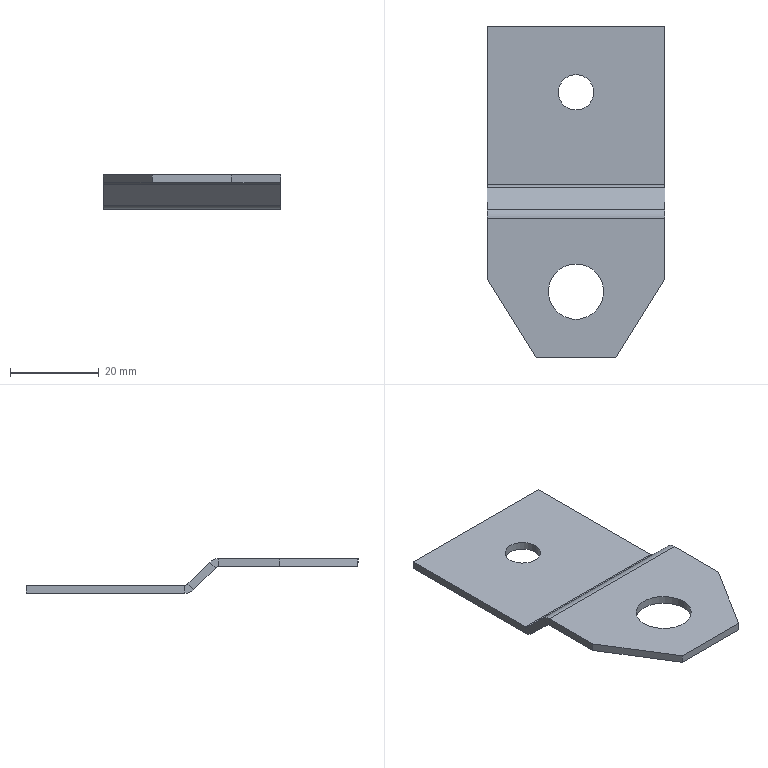Part | SolidWorks | features FlatPattern 1, Jog 1, SMBaseFlange 1, SheetMetal 1 | 1 solid | 28 faces | box 40 x 75 x 7.8 mm | volume 4907 mm3 | plane 20 | cylinder 8 | commonest cylinder face diameters 2 x2 5.6 x2 8 x2 12.5 x2
STEP:
#1=CARTESIAN_POINT('',(573.75,-25.,7.8));
#2=VERTEX_POINT('',#1);
#3=CARTESIAN_POINT('',(586.25,-25.,7.8));
#4=VERTEX_POINT('',#3);
#5=CARTESIAN_POINT('',(580.,-25.,7.8));
#6=DIRECTION('',(0.,0.,1.));
#7=DIRECTION('',(1.,0.,0.));
#8=AXIS2_PLACEMENT_3D('',#5,#6,#7);
#9=CIRCLE('',#8,6.25);
#10=EDGE_CURVE('',#2,#4,#9,.T.);
#11=ORIENTED_EDGE('',*,*,#10,.T.);
#12=CARTESIAN_POINT('',(586.25,-25.,6.));
#13=VERTEX_POINT('',#12);
#14=CARTESIAN_POINT('',(586.25,-25.,7.8));
#15=DIRECTION('',(0.,0.,-1.));
#16=VECTOR('',#15,1000.);
#17=LINE('',#14,#16);
#18=EDGE_CURVE('',#4,#13,#17,.T.);
#19=ORIENTED_EDGE('',*,*,#18,.T.);
#20=CARTESIAN_POINT('',(573.75,-25.,6.));
#21=VERTEX_POINT('',#20);
#22=CARTESIAN_POINT('',(580.,-25.,6.));
#23=DIRECTION('',(0.,0.,1.));
#24=DIRECTION('',(1.,0.,0.));
#25=AXIS2_PLACEMENT_3D('',#22,#23,#24);
#26=CIRCLE('',#25,6.25);
#27=EDGE_CURVE('',#21,#13,#26,.T.);
#28=ORIENTED_EDGE('',*,*,#27,.F.);
#29=CARTESIAN_POINT('',(573.75,-25.,7.8));
#30=DIRECTION('',(0.,0.,-1.));
#31=VECTOR('',#30,1000.);
#32=LINE('',#29,#31);
#33=EDGE_CURVE('',#2,#21,#32,.T.);
#34=ORIENTED_EDGE('',*,*,#33,.F.);
#35=EDGE_LOOP('',(#11,#19,#28,#34));
#36=FACE_OUTER_BOUND('',#35,.T.);
#37=CARTESIAN_POINT('',(580.,-25.,7.8));
#38=DIRECTION('',(0.,0.,-1.));
#39=DIRECTION('',(-1.,0.,0.));
#40=AXIS2_PLACEMENT_3D('',#37,#38,#39);
#41=CYLINDRICAL_SURFACE('',#40,6.25);
#42=ADVANCED_FACE('',(#36),#41,.F.);
#43=CARTESIAN_POINT('',(576.,20.,1.8));
#44=VERTEX_POINT('',#43);
#45=CARTESIAN_POINT('',(584.,20.,1.8));
#46=VERTEX_POINT('',#45);
#47=CARTESIAN_POINT('',(580.,20.,1.8));
#48=DIRECTION('',(0.,0.,1.));
#49=DIRECTION('',(1.,0.,0.));
#50=AXIS2_PLACEMENT_3D('',#47,#48,#49);
#51=CIRCLE('',#50,4.);
#52=EDGE_CURVE('',#44,#46,#51,.T.);
#53=ORIENTED_EDGE('',*,*,#52,.T.);
#54=CARTESIAN_POINT('',(584.,20.,0.));
#55=VERTEX_POINT('',#54);
#56=CARTESIAN_POINT('',(584.,20.,1.8));
#57=DIRECTION('',(0.,0.,-1.));
#58=VECTOR('',#57,1000.);
#59=LINE('',#56,#58);
#60=EDGE_CURVE('',#46,#55,#59,.T.);
#61=ORIENTED_EDGE('',*,*,#60,.T.);
#62=CARTESIAN_POINT('',(576.,20.,0.));
#63=VERTEX_POINT('',#62);
#64=CARTESIAN_POINT('',(580.,20.,0.));
#65=DIRECTION('',(0.,0.,1.));
#66=DIRECTION('',(1.,0.,0.));
#67=AXIS2_PLACEMENT_3D('',#64,#65,#66);
#68=CIRCLE('',#67,4.);
#69=EDGE_CURVE('',#63,#55,#68,.T.);
#70=ORIENTED_EDGE('',*,*,#69,.F.);
#71=CARTESIAN_POINT('',(576.,20.,1.8));
#72=DIRECTION('',(0.,0.,-1.));
#73=VECTOR('',#72,1000.);
#74=LINE('',#71,#73);
#75=EDGE_CURVE('',#44,#63,#74,.T.);
#76=ORIENTED_EDGE('',*,*,#75,.F.);
#77=EDGE_LOOP('',(#53,#61,#70,#76));
#78=FACE_OUTER_BOUND('',#77,.T.);
#79=CARTESIAN_POINT('',(580.,20.,1.8));
#80=DIRECTION('',(0.,0.,-1.));
#81=DIRECTION('',(-1.,0.,0.));
#82=AXIS2_PLACEMENT_3D('',#79,#80,#81);
#83=CYLINDRICAL_SURFACE('',#82,4.);
#84=ADVANCED_FACE('',(#78),#83,.F.);
#85=CARTESIAN_POINT('',(600.,-6.475,6.98));
#86=VERTEX_POINT('',#85);
#87=CARTESIAN_POINT('',(600.,-1.588,2.093));
#88=VERTEX_POINT('',#87);
#89=CARTESIAN_POINT('',(600.,24.729,-24.224));
#90=DIRECTION('',(0.,0.7071,-0.7071));
#91=VECTOR('',#90,1000.);
#92=LINE('',#89,#91);
#93=EDGE_CURVE('',#86,#88,#92,.T.);
#94=ORIENTED_EDGE('',*,*,#93,.F.);
#95=CARTESIAN_POINT('',(600.,-7.748,5.707));
#96=VERTEX_POINT('',#95);
#97=CARTESIAN_POINT('',(600.,-6.475,6.98));
#98=DIRECTION('',(0.,-0.7071,-0.7071));
#99=VECTOR('',#98,1000.);
#100=LINE('',#97,#99);
#101=EDGE_CURVE('',#86,#96,#100,.T.);
#102=ORIENTED_EDGE('',*,*,#101,.T.);
#103=CARTESIAN_POINT('',(600.,-2.861,0.8201));
#104=VERTEX_POINT('',#103);
#105=CARTESIAN_POINT('',(600.,23.456,-25.497));
#106=DIRECTION('',(0.,0.7071,-0.7071));
#107=VECTOR('',#106,1000.);
#108=LINE('',#105,#107);
#109=EDGE_CURVE('',#96,#104,#108,.T.);
#110=ORIENTED_EDGE('',*,*,#109,.T.);
#111=CARTESIAN_POINT('',(600.,-1.588,2.093));
#112=DIRECTION('',(0.,-0.7071,-0.7071));
#113=VECTOR('',#112,1000.);
#114=LINE('',#111,#113);
#115=EDGE_CURVE('',#88,#104,#114,.T.);
#116=ORIENTED_EDGE('',*,*,#115,.F.);
#117=EDGE_LOOP('',(#94,#102,#110,#116));
#118=FACE_OUTER_BOUND('',#117,.T.);
#119=CARTESIAN_POINT('',(600.,24.729,-24.224));
#120=DIRECTION('',(-1.,0.,0.));
#121=DIRECTION('',(0.,-0.7071,0.7071));
#122=AXIS2_PLACEMENT_3D('',#119,#120,#121);
#123=PLANE('',#122);
#124=ADVANCED_FACE('',(#118),#123,.F.);
#125=CARTESIAN_POINT('',(560.,-2.861,0.8201));
#126=VERTEX_POINT('',#125);
#127=CARTESIAN_POINT('',(560.,-7.748,5.707));
#128=VERTEX_POINT('',#127);
#129=CARTESIAN_POINT('',(560.,23.456,-25.497));
#130=DIRECTION('',(0.,-0.7071,0.7071));
#131=VECTOR('',#130,1000.);
#132=LINE('',#129,#131);
#133=EDGE_CURVE('',#126,#128,#132,.T.);
#134=ORIENTED_EDGE('',*,*,#133,.T.);
#135=CARTESIAN_POINT('',(560.,-6.475,6.98));
#136=VERTEX_POINT('',#135);
#137=CARTESIAN_POINT('',(560.,-6.475,6.98));
#138=DIRECTION('',(0.,0.7071,0.7071));
#139=VECTOR('',#138,1000.);
#140=LINE('',#137,#139);
#141=EDGE_CURVE('',#128,#136,#140,.T.);
#142=ORIENTED_EDGE('',*,*,#141,.T.);
#143=CARTESIAN_POINT('',(560.,-1.588,2.093));
#144=VERTEX_POINT('',#143);
#145=CARTESIAN_POINT('',(560.,24.729,-24.224));
#146=DIRECTION('',(0.,-0.7071,0.7071));
#147=VECTOR('',#146,1000.);
#148=LINE('',#145,#147);
#149=EDGE_CURVE('',#144,#136,#148,.T.);
#150=ORIENTED_EDGE('',*,*,#149,.F.);
#151=CARTESIAN_POINT('',(560.,-1.588,2.093));
#152=DIRECTION('',(0.,0.7071,0.7071));
#153=VECTOR('',#152,1000.);
#154=LINE('',#151,#153);
#155=EDGE_CURVE('',#126,#144,#154,.T.);
#156=ORIENTED_EDGE('',*,*,#155,.F.);
#157=EDGE_LOOP('',(#134,#142,#150,#156));
#158=FACE_OUTER_BOUND('',#157,.T.);
#159=CARTESIAN_POINT('',(560.,24.729,-24.224));
#160=DIRECTION('',(1.,0.,0.));
#161=DIRECTION('',(0.,0.7071,-0.7071));
#162=AXIS2_PLACEMENT_3D('',#159,#160,#161);
#163=PLANE('',#162);
#164=ADVANCED_FACE('',(#158),#163,.F.);
#165=ORIENTED_EDGE('',*,*,#149,.T.);
#166=CARTESIAN_POINT('',(560.,-6.475,6.98));
#167=DIRECTION('',(1.,0.,0.));
#168=VECTOR('',#167,1000.);
#169=LINE('',#166,#168);
#170=EDGE_CURVE('',#136,#86,#169,.T.);
#171=ORIENTED_EDGE('',*,*,#170,.T.);
#172=ORIENTED_EDGE('',*,*,#93,.T.);
#173=CARTESIAN_POINT('',(560.,-1.588,2.093));
#174=DIRECTION('',(1.,0.,0.));
#175=VECTOR('',#174,1000.);
#176=LINE('',#173,#175);
#177=EDGE_CURVE('',#144,#88,#176,.T.);
#178=ORIENTED_EDGE('',*,*,#177,.F.);
#179=EDGE_LOOP('',(#165,#171,#172,#178));
#180=FACE_OUTER_BOUND('',#179,.T.);
#181=CARTESIAN_POINT('',(560.,-28.304,28.809));
#182=DIRECTION('',(0.,-0.7071,-0.7071));
#183=DIRECTION('',(-1.,0.,0.));
#184=AXIS2_PLACEMENT_3D('',#181,#182,#183);
#185=PLANE('',#184);
#186=ADVANCED_FACE('',(#180),#185,.F.);
#187=CARTESIAN_POINT('',(560.,-7.748,5.707));
#188=DIRECTION('',(1.,0.,0.));
#189=VECTOR('',#188,1000.);
#190=LINE('',#187,#189);
#191=EDGE_CURVE('',#128,#96,#190,.T.);
#192=ORIENTED_EDGE('',*,*,#191,.F.);
#193=ORIENTED_EDGE('',*,*,#133,.F.);
#194=CARTESIAN_POINT('',(560.,-2.861,0.8201));
#195=DIRECTION('',(1.,0.,0.));
#196=VECTOR('',#195,1000.);
#197=LINE('',#194,#196);
#198=EDGE_CURVE('',#126,#104,#197,.T.);
#199=ORIENTED_EDGE('',*,*,#198,.T.);
#200=ORIENTED_EDGE('',*,*,#109,.F.);
#201=EDGE_LOOP('',(#192,#193,#199,#200));
#202=FACE_OUTER_BOUND('',#201,.T.);
#203=CARTESIAN_POINT('',(560.,-29.577,27.536));
#204=DIRECTION('',(0.,-0.7071,-0.7071));
#205=DIRECTION('',(-1.,0.,0.));
#206=AXIS2_PLACEMENT_3D('',#203,#204,#205);
#207=PLANE('',#206);
#208=ADVANCED_FACE('',(#202),#207,.T.);
#209=CARTESIAN_POINT('',(600.,35.,0.));
#210=VERTEX_POINT('',#209);
#211=CARTESIAN_POINT('',(560.,35.,0.));
#212=VERTEX_POINT('',#211);
#213=CARTESIAN_POINT('',(560.,35.,0.));
#214=DIRECTION('',(-1.,0.,0.));
#215=VECTOR('',#214,1000.);
#216=LINE('',#213,#215);
#217=EDGE_CURVE('',#210,#212,#216,.T.);
#218=ORIENTED_EDGE('',*,*,#217,.T.);
#219=CARTESIAN_POINT('',(560.,35.,1.8));
#220=VERTEX_POINT('',#219);
#221=CARTESIAN_POINT('',(560.,35.,1.8));
#222=DIRECTION('',(0.,0.,-1.));
#223=VECTOR('',#222,1000.);
#224=LINE('',#221,#223);
#225=EDGE_CURVE('',#220,#212,#224,.T.);
#226=ORIENTED_EDGE('',*,*,#225,.F.);
#227=CARTESIAN_POINT('',(600.,35.,1.8));
#228=VERTEX_POINT('',#227);
#229=CARTESIAN_POINT('',(560.,35.,1.8));
#230=DIRECTION('',(-1.,0.,0.));
#231=VECTOR('',#230,1000.);
#232=LINE('',#229,#231);
#233=EDGE_CURVE('',#228,#220,#232,.T.);
#234=ORIENTED_EDGE('',*,*,#233,.F.);
#235=CARTESIAN_POINT('',(600.,35.,1.8));
#236=DIRECTION('',(0.,0.,-1.));
#237=VECTOR('',#236,1000.);
#238=LINE('',#235,#237);
#239=EDGE_CURVE('',#228,#210,#238,.T.);
#240=ORIENTED_EDGE('',*,*,#239,.T.);
#241=EDGE_LOOP('',(#218,#226,#234,#240));
#242=FACE_OUTER_BOUND('',#241,.T.);
#243=CARTESIAN_POINT('',(560.,35.,1.8));
#244=DIRECTION('',(0.,-1.,0.));
#245=DIRECTION('',(1.,0.,0.));
#246=AXIS2_PLACEMENT_3D('',#243,#244,#245);
#247=PLANE('',#246);
#248=ADVANCED_FACE('',(#242),#247,.F.);
#249=ORIENTED_EDGE('',*,*,#60,.F.);
#250=CARTESIAN_POINT('',(580.,20.,1.8));
#251=DIRECTION('',(0.,0.,1.));
#252=DIRECTION('',(1.,0.,0.));
#253=AXIS2_PLACEMENT_3D('',#250,#251,#252);
#254=CIRCLE('',#253,4.);
#255=EDGE_CURVE('',#46,#44,#254,.T.);
#256=ORIENTED_EDGE('',*,*,#255,.T.);
#257=ORIENTED_EDGE('',*,*,#75,.T.);
#258=CARTESIAN_POINT('',(580.,20.,0.));
#259=DIRECTION('',(0.,0.,1.));
#260=DIRECTION('',(1.,0.,0.));
#261=AXIS2_PLACEMENT_3D('',#258,#259,#260);
#262=CIRCLE('',#261,4.);
#263=EDGE_CURVE('',#55,#63,#262,.T.);
#264=ORIENTED_EDGE('',*,*,#263,.F.);
#265=EDGE_LOOP('',(#249,#256,#257,#264));
#266=FACE_OUTER_BOUND('',#265,.T.);
#267=CARTESIAN_POINT('',(580.,20.,1.8));
#268=DIRECTION('',(0.,0.,-1.));
#269=DIRECTION('',(-1.,0.,0.));
#270=AXIS2_PLACEMENT_3D('',#267,#268,#269);
#271=CYLINDRICAL_SURFACE('',#270,4.);
#272=ADVANCED_FACE('',(#266),#271,.F.);
#273=ORIENTED_EDGE('',*,*,#52,.F.);
#274=ORIENTED_EDGE('',*,*,#255,.F.);
#275=EDGE_LOOP('',(#273,#274));
#276=FACE_BOUND('',#275,.T.);
#277=CARTESIAN_POINT('',(560.,-0.8814,1.8));
#278=VERTEX_POINT('',#277);
#279=CARTESIAN_POINT('',(560.,35.,1.8));
#280=DIRECTION('',(0.,-1.,0.));
#281=VECTOR('',#280,1000.);
#282=LINE('',#279,#281);
#283=EDGE_CURVE('',#220,#278,#282,.T.);
#284=ORIENTED_EDGE('',*,*,#283,.T.);
#285=CARTESIAN_POINT('',(600.,-0.8814,1.8));
#286=VERTEX_POINT('',#285);
#287=CARTESIAN_POINT('',(560.,-0.8814,1.8));
#288=DIRECTION('',(1.,0.,0.));
#289=VECTOR('',#288,1000.);
#290=LINE('',#287,#289);
#291=EDGE_CURVE('',#278,#286,#290,.T.);
#292=ORIENTED_EDGE('',*,*,#291,.T.);
#293=CARTESIAN_POINT('',(600.,35.,1.8));
#294=DIRECTION('',(0.,1.,0.));
#295=VECTOR('',#294,1000.);
#296=LINE('',#293,#295);
#297=EDGE_CURVE('',#286,#228,#296,.T.);
#298=ORIENTED_EDGE('',*,*,#297,.T.);
#299=ORIENTED_EDGE('',*,*,#233,.T.);
#300=EDGE_LOOP('',(#284,#292,#298,#299));
#301=FACE_OUTER_BOUND('',#300,.T.);
#302=CARTESIAN_POINT('',(560.,-40.,1.8));
#303=DIRECTION('',(0.,0.,-1.));
#304=DIRECTION('',(-1.,0.,0.));
#305=AXIS2_PLACEMENT_3D('',#302,#303,#304);
#306=PLANE('',#305);
#307=ADVANCED_FACE('',(#276,#301),#306,.F.);
#308=ORIENTED_EDGE('',*,*,#297,.F.);
#309=CARTESIAN_POINT('',(600.,-0.8814,0.));
#310=VERTEX_POINT('',#309);
#311=CARTESIAN_POINT('',(600.,-0.8814,1.8));
#312=DIRECTION('',(0.,0.,-1.));
#313=VECTOR('',#312,1000.);
#314=LINE('',#311,#313);
#315=EDGE_CURVE('',#286,#310,#314,.T.);
#316=ORIENTED_EDGE('',*,*,#315,.T.);
#317=CARTESIAN_POINT('',(600.,35.,0.));
#318=DIRECTION('',(0.,1.,0.));
#319=VECTOR('',#318,1000.);
#320=LINE('',#317,#319);
#321=EDGE_CURVE('',#310,#210,#320,.T.);
#322=ORIENTED_EDGE('',*,*,#321,.T.);
#323=ORIENTED_EDGE('',*,*,#239,.F.);
#324=EDGE_LOOP('',(#308,#316,#322,#323));
#325=FACE_OUTER_BOUND('',#324,.T.);
#326=CARTESIAN_POINT('',(600.,35.,1.8));
#327=DIRECTION('',(-1.,0.,0.));
#328=DIRECTION('',(0.,-1.,0.));
#329=AXIS2_PLACEMENT_3D('',#326,#327,#328);
#330=PLANE('',#329);
#331=ADVANCED_FACE('',(#325),#330,.F.);
#332=CARTESIAN_POINT('',(560.,-0.8814,0.));
#333=VERTEX_POINT('',#332);
#334=CARTESIAN_POINT('',(560.,-0.8814,0.));
#335=DIRECTION('',(1.,0.,0.));
#336=VECTOR('',#335,1000.);
#337=LINE('',#334,#336);
#338=EDGE_CURVE('',#333,#310,#337,.T.);
#339=ORIENTED_EDGE('',*,*,#338,.F.);
#340=CARTESIAN_POINT('',(560.,35.,0.));
#341=DIRECTION('',(0.,-1.,0.));
#342=VECTOR('',#341,1000.);
#343=LINE('',#340,#342);
#344=EDGE_CURVE('',#212,#333,#343,.T.);
#345=ORIENTED_EDGE('',*,*,#344,.F.);
#346=ORIENTED_EDGE('',*,*,#217,.F.);
#347=ORIENTED_EDGE('',*,*,#321,.F.);
#348=EDGE_LOOP('',(#339,#345,#346,#347));
#349=FACE_OUTER_BOUND('',#348,.T.);
#350=ORIENTED_EDGE('',*,*,#69,.T.);
#351=ORIENTED_EDGE('',*,*,#263,.T.);
#352=EDGE_LOOP('',(#350,#351));
#353=FACE_BOUND('',#352,.T.);
#354=CARTESIAN_POINT('',(560.,-40.,0.));
#355=DIRECTION('',(0.,0.,-1.));
#356=DIRECTION('',(-1.,0.,0.));
#357=AXIS2_PLACEMENT_3D('',#354,#355,#356);
#358=PLANE('',#357);
#359=ADVANCED_FACE('',(#349,#353),#358,.T.);
#360=ORIENTED_EDGE('',*,*,#344,.T.);
#361=CARTESIAN_POINT('',(560.,-0.8814,1.8));
#362=DIRECTION('',(0.,0.,1.));
#363=VECTOR('',#362,1000.);
#364=LINE('',#361,#363);
#365=EDGE_CURVE('',#333,#278,#364,.T.);
#366=ORIENTED_EDGE('',*,*,#365,.T.);
#367=ORIENTED_EDGE('',*,*,#283,.F.);
#368=ORIENTED_EDGE('',*,*,#225,.T.);
#369=EDGE_LOOP('',(#360,#366,#367,#368));
#370=FACE_OUTER_BOUND('',#369,.T.);
#371=CARTESIAN_POINT('',(560.,35.,1.8));
#372=DIRECTION('',(1.,0.,0.));
#373=DIRECTION('',(0.,1.,0.));
#374=AXIS2_PLACEMENT_3D('',#371,#372,#373);
#375=PLANE('',#374);
#376=ADVANCED_FACE('',(#370),#375,.F.);
#377=ORIENTED_EDGE('',*,*,#365,.F.);
#378=CARTESIAN_POINT('',(560.,-0.8814,2.8));
#379=DIRECTION('',(-1.,0.,0.));
#380=DIRECTION('',(0.,1.,0.));
#381=AXIS2_PLACEMENT_3D('',#378,#379,#380);
#382=CIRCLE('',#381,2.8);
#383=EDGE_CURVE('',#333,#126,#382,.T.);
#384=ORIENTED_EDGE('',*,*,#383,.T.);
#385=ORIENTED_EDGE('',*,*,#155,.T.);
#386=CARTESIAN_POINT('',(560.,-0.8814,2.8));
#387=DIRECTION('',(-1.,0.,0.));
#388=DIRECTION('',(0.,0.,1.));
#389=AXIS2_PLACEMENT_3D('',#386,#387,#388);
#390=CIRCLE('',#389,1.);
#391=EDGE_CURVE('',#278,#144,#390,.T.);
#392=ORIENTED_EDGE('',*,*,#391,.F.);
#393=EDGE_LOOP('',(#377,#384,#385,#392));
#394=FACE_OUTER_BOUND('',#393,.T.);
#395=CARTESIAN_POINT('',(560.,-0.8814,2.8));
#396=DIRECTION('',(1.,0.,0.));
#397=DIRECTION('',(0.,0.,-1.));
#398=AXIS2_PLACEMENT_3D('',#395,#396,#397);
#399=PLANE('',#398);
#400=ADVANCED_FACE('',(#394),#399,.F.);
#401=ORIENTED_EDGE('',*,*,#115,.T.);
#402=CARTESIAN_POINT('',(600.,-0.8814,2.8));
#403=DIRECTION('',(1.,0.,0.));
#404=DIRECTION('',(0.,1.,0.));
#405=AXIS2_PLACEMENT_3D('',#402,#403,#404);
#406=CIRCLE('',#405,2.8);
#407=EDGE_CURVE('',#104,#310,#406,.T.);
#408=ORIENTED_EDGE('',*,*,#407,.T.);
#409=ORIENTED_EDGE('',*,*,#315,.F.);
#410=CARTESIAN_POINT('',(600.,-0.8814,2.8));
#411=DIRECTION('',(1.,0.,0.));
#412=DIRECTION('',(0.,0.,-1.));
#413=AXIS2_PLACEMENT_3D('',#410,#411,#412);
#414=CIRCLE('',#413,1.);
#415=EDGE_CURVE('',#88,#286,#414,.T.);
#416=ORIENTED_EDGE('',*,*,#415,.F.);
#417=EDGE_LOOP('',(#401,#408,#409,#416));
#418=FACE_OUTER_BOUND('',#417,.T.);
#419=CARTESIAN_POINT('',(600.,-0.8814,2.8));
#420=DIRECTION('',(-1.,0.,0.));
#421=DIRECTION('',(0.,0.,1.));
#422=AXIS2_PLACEMENT_3D('',#419,#420,#421);
#423=PLANE('',#422);
#424=ADVANCED_FACE('',(#418),#423,.F.);
#425=ORIENTED_EDGE('',*,*,#415,.T.);
#426=ORIENTED_EDGE('',*,*,#291,.F.);
#427=ORIENTED_EDGE('',*,*,#391,.T.);
#428=ORIENTED_EDGE('',*,*,#177,.T.);
#429=EDGE_LOOP('',(#425,#426,#427,#428));
#430=FACE_OUTER_BOUND('',#429,.T.);
#431=CARTESIAN_POINT('',(539.937,-0.8814,2.8));
#432=DIRECTION('',(1.,0.,0.));
#433=DIRECTION('',(0.,1.,0.));
#434=AXIS2_PLACEMENT_3D('',#431,#432,#433);
#435=CYLINDRICAL_SURFACE('',#434,1.);
#436=ADVANCED_FACE('',(#430),#435,.F.);
#437=ORIENTED_EDGE('',*,*,#407,.F.);
#438=ORIENTED_EDGE('',*,*,#198,.F.);
#439=ORIENTED_EDGE('',*,*,#383,.F.);
#440=ORIENTED_EDGE('',*,*,#338,.T.);
#441=EDGE_LOOP('',(#437,#438,#439,#440));
#442=FACE_OUTER_BOUND('',#441,.T.);
#443=CARTESIAN_POINT('',(539.937,-0.8814,2.8));
#444=DIRECTION('',(1.,0.,0.));
#445=DIRECTION('',(0.,1.,0.));
#446=AXIS2_PLACEMENT_3D('',#443,#444,#445);
#447=CYLINDRICAL_SURFACE('',#446,2.8);
#448=ADVANCED_FACE('',(#442),#447,.T.);
#449=ORIENTED_EDGE('',*,*,#141,.F.);
#450=CARTESIAN_POINT('',(560.,-8.455,6.));
#451=VERTEX_POINT('',#450);
#452=CARTESIAN_POINT('',(560.,-8.455,5.));
#453=DIRECTION('',(1.,0.,0.));
#454=DIRECTION('',(0.,1.,0.));
#455=AXIS2_PLACEMENT_3D('',#452,#453,#454);
#456=CIRCLE('',#455,1.);
#457=EDGE_CURVE('',#128,#451,#456,.T.);
#458=ORIENTED_EDGE('',*,*,#457,.T.);
#459=CARTESIAN_POINT('',(560.,-8.455,7.8));
#460=VERTEX_POINT('',#459);
#461=CARTESIAN_POINT('',(560.,-8.455,7.8));
#462=DIRECTION('',(0.,0.,1.));
#463=VECTOR('',#462,1000.);
#464=LINE('',#461,#463);
#465=EDGE_CURVE('',#451,#460,#464,.T.);
#466=ORIENTED_EDGE('',*,*,#465,.T.);
#467=CARTESIAN_POINT('',(560.,-8.455,5.));
#468=DIRECTION('',(1.,0.,0.));
#469=DIRECTION('',(0.,0.,-1.));
#470=AXIS2_PLACEMENT_3D('',#467,#468,#469);
#471=CIRCLE('',#470,2.8);
#472=EDGE_CURVE('',#136,#460,#471,.T.);
#473=ORIENTED_EDGE('',*,*,#472,.F.);
#474=EDGE_LOOP('',(#449,#458,#466,#473));
#475=FACE_OUTER_BOUND('',#474,.T.);
#476=CARTESIAN_POINT('',(560.,-8.455,5.));
#477=DIRECTION('',(-1.,0.,0.));
#478=DIRECTION('',(0.,0.,1.));
#479=AXIS2_PLACEMENT_3D('',#476,#477,#478);
#480=PLANE('',#479);
#481=ADVANCED_FACE('',(#475),#480,.T.);
#482=CARTESIAN_POINT('',(600.,-8.455,7.8));
#483=VERTEX_POINT('',#482);
#484=CARTESIAN_POINT('',(600.,-8.455,6.));
#485=VERTEX_POINT('',#484);
#486=CARTESIAN_POINT('',(600.,-8.455,7.8));
#487=DIRECTION('',(0.,0.,-1.));
#488=VECTOR('',#487,1000.);
#489=LINE('',#486,#488);
#490=EDGE_CURVE('',#483,#485,#489,.T.);
#491=ORIENTED_EDGE('',*,*,#490,.T.);
#492=CARTESIAN_POINT('',(600.,-8.455,5.));
#493=DIRECTION('',(-1.,0.,0.));
#494=DIRECTION('',(0.,1.,0.));
#495=AXIS2_PLACEMENT_3D('',#492,#493,#494);
#496=CIRCLE('',#495,1.);
#497=EDGE_CURVE('',#485,#96,#496,.T.);
#498=ORIENTED_EDGE('',*,*,#497,.T.);
#499=ORIENTED_EDGE('',*,*,#101,.F.);
#500=CARTESIAN_POINT('',(600.,-8.455,5.));
#501=DIRECTION('',(-1.,0.,0.));
#502=DIRECTION('',(0.,0.,1.));
#503=AXIS2_PLACEMENT_3D('',#500,#501,#502);
#504=CIRCLE('',#503,2.8);
#505=EDGE_CURVE('',#483,#86,#504,.T.);
#506=ORIENTED_EDGE('',*,*,#505,.F.);
#507=EDGE_LOOP('',(#491,#498,#499,#506));
#508=FACE_OUTER_BOUND('',#507,.T.);
#509=CARTESIAN_POINT('',(600.,-8.455,5.));
#510=DIRECTION('',(1.,0.,0.));
#511=DIRECTION('',(0.,0.,-1.));
#512=AXIS2_PLACEMENT_3D('',#509,#510,#511);
#513=PLANE('',#512);
#514=ADVANCED_FACE('',(#508),#513,.T.);
#515=ORIENTED_EDGE('',*,*,#505,.T.);
#516=ORIENTED_EDGE('',*,*,#170,.F.);
#517=ORIENTED_EDGE('',*,*,#472,.T.);
#518=CARTESIAN_POINT('',(560.,-8.455,7.8));
#519=DIRECTION('',(1.,0.,0.));
#520=VECTOR('',#519,1000.);
#521=LINE('',#518,#520);
#522=EDGE_CURVE('',#460,#483,#521,.T.);
#523=ORIENTED_EDGE('',*,*,#522,.T.);
#524=EDGE_LOOP('',(#515,#516,#517,#523));
#525=FACE_OUTER_BOUND('',#524,.T.);
#526=CARTESIAN_POINT('',(539.877,-8.455,5.));
#527=DIRECTION('',(1.,0.,0.));
#528=DIRECTION('',(0.,1.,0.));
#529=AXIS2_PLACEMENT_3D('',#526,#527,#528);
#530=CYLINDRICAL_SURFACE('',#529,2.8);
#531=ADVANCED_FACE('',(#525),#530,.T.);
#532=ORIENTED_EDGE('',*,*,#497,.F.);
#533=CARTESIAN_POINT('',(560.,-8.455,6.));
#534=DIRECTION('',(1.,0.,0.));
#535=VECTOR('',#534,1000.);
#536=LINE('',#533,#535);
#537=EDGE_CURVE('',#451,#485,#536,.T.);
#538=ORIENTED_EDGE('',*,*,#537,.F.);
#539=ORIENTED_EDGE('',*,*,#457,.F.);
#540=ORIENTED_EDGE('',*,*,#191,.T.);
#541=EDGE_LOOP('',(#532,#538,#539,#540));
#542=FACE_OUTER_BOUND('',#541,.T.);
#543=CARTESIAN_POINT('',(539.877,-8.455,5.));
#544=DIRECTION('',(1.,0.,0.));
#545=DIRECTION('',(0.,1.,0.));
#546=AXIS2_PLACEMENT_3D('',#543,#544,#545);
#547=CYLINDRICAL_SURFACE('',#546,1.);
#548=ADVANCED_FACE('',(#542),#547,.F.);
#549=ORIENTED_EDGE('',*,*,#18,.F.);
#550=CARTESIAN_POINT('',(580.,-25.,7.8));
#551=DIRECTION('',(0.,0.,1.));
#552=DIRECTION('',(1.,0.,0.));
#553=AXIS2_PLACEMENT_3D('',#550,#551,#552);
#554=CIRCLE('',#553,6.25);
#555=EDGE_CURVE('',#4,#2,#554,.T.);
#556=ORIENTED_EDGE('',*,*,#555,.T.);
#557=ORIENTED_EDGE('',*,*,#33,.T.);
#558=CARTESIAN_POINT('',(580.,-25.,6.));
#559=DIRECTION('',(0.,0.,1.));
#560=DIRECTION('',(1.,0.,0.));
#561=AXIS2_PLACEMENT_3D('',#558,#559,#560);
#562=CIRCLE('',#561,6.25);
#563=EDGE_CURVE('',#13,#21,#562,.T.);
#564=ORIENTED_EDGE('',*,*,#563,.F.);
#565=EDGE_LOOP('',(#549,#556,#557,#564));
#566=FACE_OUTER_BOUND('',#565,.T.);
#567=CARTESIAN_POINT('',(580.,-25.,7.8));
#568=DIRECTION('',(0.,0.,-1.));
#569=DIRECTION('',(-1.,0.,0.));
#570=AXIS2_PLACEMENT_3D('',#567,#568,#569);
#571=CYLINDRICAL_SURFACE('',#570,6.25);
#572=ADVANCED_FACE('',(#566),#571,.F.);
#573=CARTESIAN_POINT('',(589.,-40.,6.));
#574=VERTEX_POINT('',#573);
#575=CARTESIAN_POINT('',(600.,-22.365,6.));
#576=VERTEX_POINT('',#575);
#577=CARTESIAN_POINT('',(589.,-40.,6.));
#578=DIRECTION('',(0.5292,0.8485,0.));
#579=VECTOR('',#578,1000.);
#580=LINE('',#577,#579);
#581=EDGE_CURVE('',#574,#576,#580,.T.);
#582=ORIENTED_EDGE('',*,*,#581,.T.);
#583=CARTESIAN_POINT('',(600.,-22.365,7.8));
#584=VERTEX_POINT('',#583);
#585=CARTESIAN_POINT('',(600.,-22.365,7.8));
#586=DIRECTION('',(0.,0.,-1.));
#587=VECTOR('',#586,1000.);
#588=LINE('',#585,#587);
#589=EDGE_CURVE('',#584,#576,#588,.T.);
#590=ORIENTED_EDGE('',*,*,#589,.F.);
#591=CARTESIAN_POINT('',(589.,-40.,7.8));
#592=VERTEX_POINT('',#591);
#593=CARTESIAN_POINT('',(589.,-40.,7.8));
#594=DIRECTION('',(0.5292,0.8485,0.));
#595=VECTOR('',#594,1000.);
#596=LINE('',#593,#595);
#597=EDGE_CURVE('',#592,#584,#596,.T.);
#598=ORIENTED_EDGE('',*,*,#597,.F.);
#599=CARTESIAN_POINT('',(589.,-40.,7.8));
#600=DIRECTION('',(0.,0.,-1.));
#601=VECTOR('',#600,1000.);
#602=LINE('',#599,#601);
#603=EDGE_CURVE('',#592,#574,#602,.T.);
#604=ORIENTED_EDGE('',*,*,#603,.T.);
#605=EDGE_LOOP('',(#582,#590,#598,#604));
#606=FACE_OUTER_BOUND('',#605,.T.);
#607=CARTESIAN_POINT('',(589.,-40.,7.8));
#608=DIRECTION('',(-0.8485,0.5292,0.));
#609=DIRECTION('',(-0.5292,-0.8485,0.));
#610=AXIS2_PLACEMENT_3D('',#607,#608,#609);
#611=PLANE('',#610);
#612=ADVANCED_FACE('',(#606),#611,.F.);
#613=CARTESIAN_POINT('',(571.,-40.,6.));
#614=VERTEX_POINT('',#613);
#615=CARTESIAN_POINT('',(589.,-40.,6.));
#616=DIRECTION('',(1.,0.,0.));
#617=VECTOR('',#616,1000.);
#618=LINE('',#615,#617);
#619=EDGE_CURVE('',#614,#574,#618,.T.);
#620=ORIENTED_EDGE('',*,*,#619,.T.);
#621=ORIENTED_EDGE('',*,*,#603,.F.);
#622=CARTESIAN_POINT('',(571.,-40.,7.8));
#623=VERTEX_POINT('',#622);
#624=CARTESIAN_POINT('',(589.,-40.,7.8));
#625=DIRECTION('',(1.,0.,0.));
#626=VECTOR('',#625,1000.);
#627=LINE('',#624,#626);
#628=EDGE_CURVE('',#623,#592,#627,.T.);
#629=ORIENTED_EDGE('',*,*,#628,.F.);
#630=CARTESIAN_POINT('',(571.,-40.,7.8));
#631=DIRECTION('',(0.,0.,-1.));
#632=VECTOR('',#631,1000.);
#633=LINE('',#630,#632);
#634=EDGE_CURVE('',#623,#614,#633,.T.);
#635=ORIENTED_EDGE('',*,*,#634,.T.);
#636=EDGE_LOOP('',(#620,#621,#629,#635));
#637=FACE_OUTER_BOUND('',#636,.T.);
#638=CARTESIAN_POINT('',(589.,-40.,7.8));
#639=DIRECTION('',(0.,1.,0.));
#640=DIRECTION('',(0.,0.,1.));
#641=AXIS2_PLACEMENT_3D('',#638,#639,#640);
#642=PLANE('',#641);
#643=ADVANCED_FACE('',(#637),#642,.F.);
#644=CARTESIAN_POINT('',(560.,-22.365,6.));
#645=VERTEX_POINT('',#644);
#646=CARTESIAN_POINT('',(571.,-40.,6.));
#647=DIRECTION('',(0.5292,-0.8485,0.));
#648=VECTOR('',#647,1000.);
#649=LINE('',#646,#648);
#650=EDGE_CURVE('',#645,#614,#649,.T.);
#651=ORIENTED_EDGE('',*,*,#650,.T.);
#652=ORIENTED_EDGE('',*,*,#634,.F.);
#653=CARTESIAN_POINT('',(560.,-22.365,7.8));
#654=VERTEX_POINT('',#653);
#655=CARTESIAN_POINT('',(571.,-40.,7.8));
#656=DIRECTION('',(0.5292,-0.8485,0.));
#657=VECTOR('',#656,1000.);
#658=LINE('',#655,#657);
#659=EDGE_CURVE('',#654,#623,#658,.T.);
#660=ORIENTED_EDGE('',*,*,#659,.F.);
#661=CARTESIAN_POINT('',(560.,-22.365,7.8));
#662=DIRECTION('',(0.,0.,-1.));
#663=VECTOR('',#662,1000.);
#664=LINE('',#661,#663);
#665=EDGE_CURVE('',#654,#645,#664,.T.);
#666=ORIENTED_EDGE('',*,*,#665,.T.);
#667=EDGE_LOOP('',(#651,#652,#660,#666));
#668=FACE_OUTER_BOUND('',#667,.T.);
#669=CARTESIAN_POINT('',(571.,-40.,7.8));
#670=DIRECTION('',(0.8485,0.5292,0.));
#671=DIRECTION('',(-0.5292,0.8485,0.));
#672=AXIS2_PLACEMENT_3D('',#669,#670,#671);
#673=PLANE('',#672);
#674=ADVANCED_FACE('',(#668),#673,.F.);
#675=ORIENTED_EDGE('',*,*,#522,.F.);
#676=CARTESIAN_POINT('',(560.,37.011,7.8));
#677=DIRECTION('',(0.,-1.,0.));
#678=VECTOR('',#677,1000.);
#679=LINE('',#676,#678);
#680=EDGE_CURVE('',#460,#654,#679,.T.);
#681=ORIENTED_EDGE('',*,*,#680,.T.);
#682=ORIENTED_EDGE('',*,*,#659,.T.);
#683=ORIENTED_EDGE('',*,*,#628,.T.);
#684=ORIENTED_EDGE('',*,*,#597,.T.);
#685=CARTESIAN_POINT('',(600.,37.011,7.8));
#686=DIRECTION('',(0.,1.,0.));
#687=VECTOR('',#686,1000.);
#688=LINE('',#685,#687);
#689=EDGE_CURVE('',#584,#483,#688,.T.);
#690=ORIENTED_EDGE('',*,*,#689,.T.);
#691=EDGE_LOOP('',(#675,#681,#682,#683,#684,#690));
#692=FACE_OUTER_BOUND('',#691,.T.);
#693=ORIENTED_EDGE('',*,*,#10,.F.);
#694=ORIENTED_EDGE('',*,*,#555,.F.);
#695=EDGE_LOOP('',(#693,#694));
#696=FACE_BOUND('',#695,.T.);
#697=CARTESIAN_POINT('',(560.,-37.989,7.8));
#698=DIRECTION('',(0.,0.,-1.));
#699=DIRECTION('',(-1.,0.,0.));
#700=AXIS2_PLACEMENT_3D('',#697,#698,#699);
#701=PLANE('',#700);
#702=ADVANCED_FACE('',(#692,#696),#701,.F.);
#703=ORIENTED_EDGE('',*,*,#465,.F.);
#704=CARTESIAN_POINT('',(560.,37.011,6.));
#705=DIRECTION('',(0.,-1.,0.));
#706=VECTOR('',#705,1000.);
#707=LINE('',#704,#706);
#708=EDGE_CURVE('',#451,#645,#707,.T.);
#709=ORIENTED_EDGE('',*,*,#708,.T.);
#710=ORIENTED_EDGE('',*,*,#665,.F.);
#711=ORIENTED_EDGE('',*,*,#680,.F.);
#712=EDGE_LOOP('',(#703,#709,#710,#711));
#713=FACE_OUTER_BOUND('',#712,.T.);
#714=CARTESIAN_POINT('',(560.,37.011,7.8));
#715=DIRECTION('',(1.,0.,0.));
#716=DIRECTION('',(0.,1.,0.));
#717=AXIS2_PLACEMENT_3D('',#714,#715,#716);
#718=PLANE('',#717);
#719=ADVANCED_FACE('',(#713),#718,.F.);
#720=ORIENTED_EDGE('',*,*,#27,.T.);
#721=ORIENTED_EDGE('',*,*,#563,.T.);
#722=EDGE_LOOP('',(#720,#721));
#723=FACE_BOUND('',#722,.T.);
#724=ORIENTED_EDGE('',*,*,#708,.F.);
#725=ORIENTED_EDGE('',*,*,#537,.T.);
#726=CARTESIAN_POINT('',(600.,37.011,6.));
#727=DIRECTION('',(0.,1.,0.));
#728=VECTOR('',#727,1000.);
#729=LINE('',#726,#728);
#730=EDGE_CURVE('',#576,#485,#729,.T.);
#731=ORIENTED_EDGE('',*,*,#730,.F.);
#732=ORIENTED_EDGE('',*,*,#581,.F.);
#733=ORIENTED_EDGE('',*,*,#619,.F.);
#734=ORIENTED_EDGE('',*,*,#650,.F.);
#735=EDGE_LOOP('',(#724,#725,#731,#732,#733,#734));
#736=FACE_OUTER_BOUND('',#735,.T.);
#737=CARTESIAN_POINT('',(560.,-37.989,6.));
#738=DIRECTION('',(0.,0.,-1.));
#739=DIRECTION('',(-1.,0.,0.));
#740=AXIS2_PLACEMENT_3D('',#737,#738,#739);
#741=PLANE('',#740);
#742=ADVANCED_FACE('',(#723,#736),#741,.T.);
#743=ORIENTED_EDGE('',*,*,#490,.F.);
#744=ORIENTED_EDGE('',*,*,#689,.F.);
#745=ORIENTED_EDGE('',*,*,#589,.T.);
#746=ORIENTED_EDGE('',*,*,#730,.T.);
#747=EDGE_LOOP('',(#743,#744,#745,#746));
#748=FACE_OUTER_BOUND('',#747,.T.);
#749=CARTESIAN_POINT('',(600.,37.011,7.8));
#750=DIRECTION('',(-1.,0.,0.));
#751=DIRECTION('',(0.,-1.,0.));
#752=AXIS2_PLACEMENT_3D('',#749,#750,#751);
#753=PLANE('',#752);
#754=ADVANCED_FACE('',(#748),#753,.F.);
#755=CLOSED_SHELL('',(#42,#84,#124,#164,#186,#208,#248,#272,#307,#331,#359,#376,#400,#424,#436,#448,#481,#514,#531,#548,#572,#612,#643,#674,#702,#719,#742,#754));
#756=MANIFOLD_SOLID_BREP('',#755);
#757=CARTESIAN_POINT('',(0.,0.,0.));
#758=DIRECTION('',(0.,0.,1.));
#759=DIRECTION('',(1.,0.,0.));
#760=AXIS2_PLACEMENT_3D('',#757,#758,#759);
#761=(LENGTH_UNIT()NAMED_UNIT(*)SI_UNIT(.MILLI.,.METRE.));
#762=UNCERTAINTY_MEASURE_WITH_UNIT(LENGTH_MEASURE(0.00001),#761,'','');
#763=(NAMED_UNIT(*)PLANE_ANGLE_UNIT()SI_UNIT($,.RADIAN.));
#764=(NAMED_UNIT(*)SI_UNIT($,.STERADIAN.)SOLID_ANGLE_UNIT());
#765=(GEOMETRIC_REPRESENTATION_CONTEXT(3)GLOBAL_UNCERTAINTY_ASSIGNED_CONTEXT((#762))GLOBAL_UNIT_ASSIGNED_CONTEXT((#761,#763,#764))REPRESENTATION_CONTEXT('',''));
#766=ADVANCED_BREP_SHAPE_REPRESENTATION('',(#756,#760),#765);